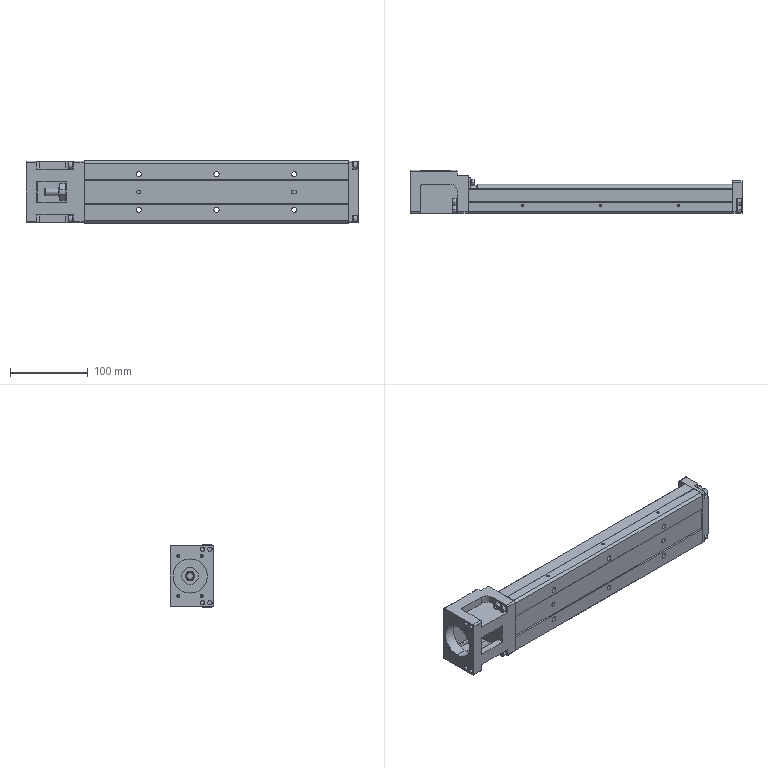Part | STEP file | Guide wheel mechanism revised.sldasm-Part-416 | 1 solid | 449 faces | box 427 x 56 x 80 mm | volume 741710 mm3 | plane 227 | cylinder 166 | cone 54 | torus 2 | commonest cylinder face diameters 4 x17 8.3 x16 8.5 x16 2.459 x12 6.6 x12 11 x12